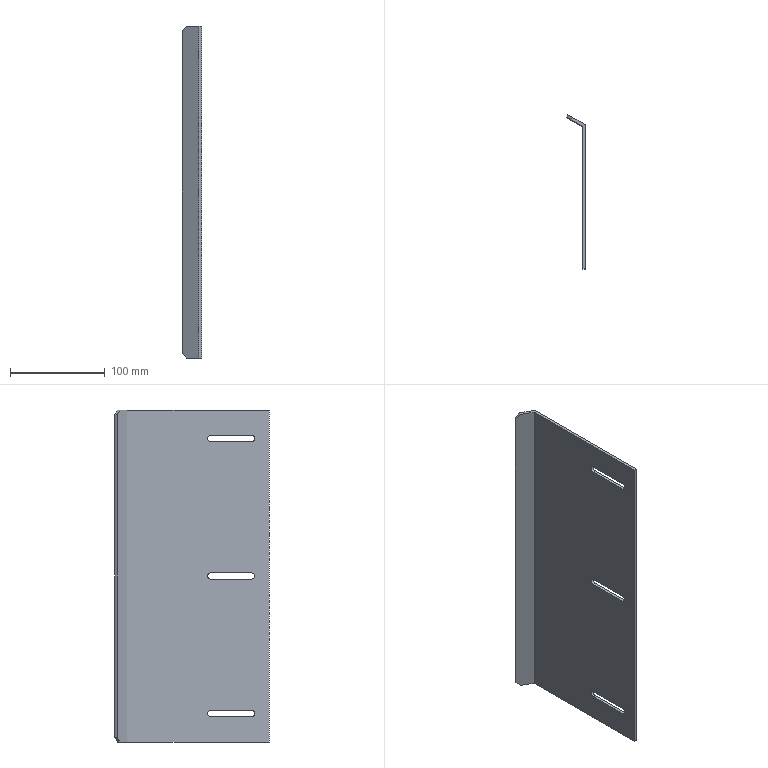Part | SolidWorks | features ICE 3, Fillet 2, Chamfer 1, Extrusion 1 | 1 solid | 24 faces | box 20.321 x 162.598 x 350 mm | volume 177208 mm3 | plane 16 | cylinder 8 | commonest cylinder face diameters 6.5 x6 0.4 x1 6.4 x1
STEP:
#1=CARTESIAN_POINT('',(0.,-150.,350.));
#2=VERTEX_POINT('',#1);
#3=CARTESIAN_POINT('',(3.,-150.,350.));
#4=VERTEX_POINT('',#3);
#5=CARTESIAN_POINT('',(0.,-150.,350.));
#6=DIRECTION('',(1.,0.,0.));
#7=VECTOR('',#6,1000.);
#8=LINE('',#5,#7);
#9=EDGE_CURVE('',#2,#4,#8,.T.);
#10=ORIENTED_EDGE('',*,*,#9,.F.);
#11=CARTESIAN_POINT('',(0.,-150.,0.));
#12=VERTEX_POINT('',#11);
#13=CARTESIAN_POINT('',(0.,-150.,0.));
#14=DIRECTION('',(0.,0.,1.));
#15=VECTOR('',#14,1000.);
#16=LINE('',#13,#15);
#17=EDGE_CURVE('',#12,#2,#16,.T.);
#18=ORIENTED_EDGE('',*,*,#17,.F.);
#19=CARTESIAN_POINT('',(3.,-150.,0.));
#20=VERTEX_POINT('',#19);
#21=CARTESIAN_POINT('',(0.,-150.,0.));
#22=DIRECTION('',(1.,0.,0.));
#23=VECTOR('',#22,1000.);
#24=LINE('',#21,#23);
#25=EDGE_CURVE('',#12,#20,#24,.T.);
#26=ORIENTED_EDGE('',*,*,#25,.T.);
#27=CARTESIAN_POINT('',(3.,-150.,0.));
#28=DIRECTION('',(0.,0.,1.));
#29=VECTOR('',#28,1000.);
#30=LINE('',#27,#29);
#31=EDGE_CURVE('',#20,#4,#30,.T.);
#32=ORIENTED_EDGE('',*,*,#31,.T.);
#33=EDGE_LOOP('',(#10,#18,#26,#32));
#34=FACE_OUTER_BOUND('',#33,.T.);
#35=CARTESIAN_POINT('',(0.,-150.,0.));
#36=DIRECTION('',(0.,-1.,0.));
#37=DIRECTION('',(0.,0.,-1.));
#38=AXIS2_PLACEMENT_3D('',#35,#36,#37);
#39=PLANE('',#38);
#40=ADVANCED_FACE('',(#34),#39,.T.);
#41=CARTESIAN_POINT('',(0.,-131.75,171.75));
#42=VERTEX_POINT('',#41);
#43=CARTESIAN_POINT('',(0.,-131.75,178.25));
#44=VERTEX_POINT('',#43);
#45=CARTESIAN_POINT('',(0.,-131.75,175.));
#46=DIRECTION('',(-1.,0.,0.));
#47=DIRECTION('',(0.,0.,1.));
#48=AXIS2_PLACEMENT_3D('',#45,#46,#47);
#49=CIRCLE('',#48,3.25);
#50=EDGE_CURVE('',#42,#44,#49,.T.);
#51=ORIENTED_EDGE('',*,*,#50,.F.);
#52=CARTESIAN_POINT('',(0.,-88.25,171.75));
#53=VERTEX_POINT('',#52);
#54=CARTESIAN_POINT('',(0.,0.,171.75));
#55=DIRECTION('',(0.,-1.,0.));
#56=VECTOR('',#55,1000.);
#57=LINE('',#54,#56);
#58=EDGE_CURVE('',#53,#42,#57,.T.);
#59=ORIENTED_EDGE('',*,*,#58,.F.);
#60=CARTESIAN_POINT('',(0.,-88.25,178.25));
#61=VERTEX_POINT('',#60);
#62=CARTESIAN_POINT('',(0.,-88.25,175.));
#63=DIRECTION('',(-1.,0.,0.));
#64=DIRECTION('',(0.,0.,1.));
#65=AXIS2_PLACEMENT_3D('',#62,#63,#64);
#66=CIRCLE('',#65,3.25);
#67=EDGE_CURVE('',#61,#53,#66,.T.);
#68=ORIENTED_EDGE('',*,*,#67,.F.);
#69=CARTESIAN_POINT('',(0.,0.,178.25));
#70=DIRECTION('',(0.,1.,0.));
#71=VECTOR('',#70,1000.);
#72=LINE('',#69,#71);
#73=EDGE_CURVE('',#44,#61,#72,.T.);
#74=ORIENTED_EDGE('',*,*,#73,.F.);
#75=EDGE_LOOP('',(#51,#59,#68,#74));
#76=FACE_BOUND('',#75,.T.);
#77=CARTESIAN_POINT('',(0.,-88.25,33.25));
#78=VERTEX_POINT('',#77);
#79=CARTESIAN_POINT('',(0.,-88.25,26.75));
#80=VERTEX_POINT('',#79);
#81=CARTESIAN_POINT('',(0.,-88.25,30.));
#82=DIRECTION('',(-1.,0.,0.));
#83=DIRECTION('',(0.,0.,1.));
#84=AXIS2_PLACEMENT_3D('',#81,#82,#83);
#85=CIRCLE('',#84,3.25);
#86=EDGE_CURVE('',#78,#80,#85,.T.);
#87=ORIENTED_EDGE('',*,*,#86,.F.);
#88=CARTESIAN_POINT('',(0.,-131.75,33.25));
#89=VERTEX_POINT('',#88);
#90=CARTESIAN_POINT('',(0.,-131.75,33.25));
#91=DIRECTION('',(0.,1.,0.));
#92=VECTOR('',#91,1000.);
#93=LINE('',#90,#92);
#94=EDGE_CURVE('',#89,#78,#93,.T.);
#95=ORIENTED_EDGE('',*,*,#94,.F.);
#96=CARTESIAN_POINT('',(0.,-131.75,26.75));
#97=VERTEX_POINT('',#96);
#98=CARTESIAN_POINT('',(0.,-131.75,30.));
#99=DIRECTION('',(-1.,0.,0.));
#100=DIRECTION('',(0.,0.,1.));
#101=AXIS2_PLACEMENT_3D('',#98,#99,#100);
#102=CIRCLE('',#101,3.25);
#103=EDGE_CURVE('',#97,#89,#102,.T.);
#104=ORIENTED_EDGE('',*,*,#103,.F.);
#105=CARTESIAN_POINT('',(0.,-88.25,26.75));
#106=DIRECTION('',(0.,-1.,0.));
#107=VECTOR('',#106,1000.);
#108=LINE('',#105,#107);
#109=EDGE_CURVE('',#80,#97,#108,.T.);
#110=ORIENTED_EDGE('',*,*,#109,.F.);
#111=EDGE_LOOP('',(#87,#95,#104,#110));
#112=FACE_BOUND('',#111,.T.);
#113=CARTESIAN_POINT('',(0.,-88.25,323.25));
#114=VERTEX_POINT('',#113);
#115=CARTESIAN_POINT('',(0.,-88.25,316.75));
#116=VERTEX_POINT('',#115);
#117=CARTESIAN_POINT('',(0.,-88.25,320.));
#118=DIRECTION('',(-1.,0.,0.));
#119=DIRECTION('',(0.,0.,1.));
#120=AXIS2_PLACEMENT_3D('',#117,#118,#119);
#121=CIRCLE('',#120,3.25);
#122=EDGE_CURVE('',#114,#116,#121,.T.);
#123=ORIENTED_EDGE('',*,*,#122,.F.);
#124=CARTESIAN_POINT('',(0.,-131.75,323.25));
#125=VERTEX_POINT('',#124);
#126=CARTESIAN_POINT('',(0.,-131.75,323.25));
#127=DIRECTION('',(0.,1.,0.));
#128=VECTOR('',#127,1000.);
#129=LINE('',#126,#128);
#130=EDGE_CURVE('',#125,#114,#129,.T.);
#131=ORIENTED_EDGE('',*,*,#130,.F.);
#132=CARTESIAN_POINT('',(0.,-131.75,316.75));
#133=VERTEX_POINT('',#132);
#134=CARTESIAN_POINT('',(0.,-131.75,320.));
#135=DIRECTION('',(-1.,0.,0.));
#136=DIRECTION('',(0.,0.,1.));
#137=AXIS2_PLACEMENT_3D('',#134,#135,#136);
#138=CIRCLE('',#137,3.25);
#139=EDGE_CURVE('',#133,#125,#138,.T.);
#140=ORIENTED_EDGE('',*,*,#139,.F.);
#141=CARTESIAN_POINT('',(0.,-88.25,316.75));
#142=DIRECTION('',(0.,-1.,0.));
#143=VECTOR('',#142,1000.);
#144=LINE('',#141,#143);
#145=EDGE_CURVE('',#116,#133,#144,.T.);
#146=ORIENTED_EDGE('',*,*,#145,.F.);
#147=EDGE_LOOP('',(#123,#131,#140,#146));
#148=FACE_BOUND('',#147,.T.);
#149=CARTESIAN_POINT('',(0.,-0.1155,350.));
#150=VERTEX_POINT('',#149);
#151=CARTESIAN_POINT('',(0.,0.,350.));
#152=DIRECTION('',(0.,-1.,0.));
#153=VECTOR('',#152,1000.);
#154=LINE('',#151,#153);
#155=EDGE_CURVE('',#150,#2,#154,.T.);
#156=ORIENTED_EDGE('',*,*,#155,.F.);
#157=CARTESIAN_POINT('',(0.,-0.1155,0.));
#158=VERTEX_POINT('',#157);
#159=CARTESIAN_POINT('',(0.,-0.1155,0.));
#160=DIRECTION('',(0.,0.,-1.));
#161=VECTOR('',#160,1000.);
#162=LINE('',#159,#161);
#163=EDGE_CURVE('',#150,#158,#162,.T.);
#164=ORIENTED_EDGE('',*,*,#163,.T.);
#165=CARTESIAN_POINT('',(0.,0.,0.));
#166=DIRECTION('',(0.,-1.,0.));
#167=VECTOR('',#166,1000.);
#168=LINE('',#165,#167);
#169=EDGE_CURVE('',#158,#12,#168,.T.);
#170=ORIENTED_EDGE('',*,*,#169,.T.);
#171=ORIENTED_EDGE('',*,*,#17,.T.);
#172=EDGE_LOOP('',(#156,#164,#170,#171));
#173=FACE_OUTER_BOUND('',#172,.T.);
#174=CARTESIAN_POINT('',(0.,0.,0.));
#175=DIRECTION('',(-1.,0.,0.));
#176=DIRECTION('',(0.,0.,1.));
#177=AXIS2_PLACEMENT_3D('',#174,#175,#176);
#178=PLANE('',#177);
#179=ADVANCED_FACE('',(#76,#112,#148,#173),#178,.T.);
#180=CARTESIAN_POINT('',(-12.99,7.5,0.));
#181=VERTEX_POINT('',#180);
#182=CARTESIAN_POINT('',(-0.1,0.05774,0.));
#183=VERTEX_POINT('',#182);
#184=CARTESIAN_POINT('',(-17.321,10.,0.));
#185=DIRECTION('',(0.866,-0.5,0.));
#186=VECTOR('',#185,1000.);
#187=LINE('',#184,#186);
#188=EDGE_CURVE('',#181,#183,#187,.T.);
#189=ORIENTED_EDGE('',*,*,#188,.T.);
#190=CARTESIAN_POINT('',(-0.1,0.05774,350.));
#191=VERTEX_POINT('',#190);
#192=CARTESIAN_POINT('',(-0.1,0.05774,350.));
#193=DIRECTION('',(0.,0.,1.));
#194=VECTOR('',#193,1000.);
#195=LINE('',#192,#194);
#196=EDGE_CURVE('',#183,#191,#195,.T.);
#197=ORIENTED_EDGE('',*,*,#196,.T.);
#198=CARTESIAN_POINT('',(-12.99,7.5,350.));
#199=VERTEX_POINT('',#198);
#200=CARTESIAN_POINT('',(-17.321,10.,350.));
#201=DIRECTION('',(0.866,-0.5,0.));
#202=VECTOR('',#201,1000.);
#203=LINE('',#200,#202);
#204=EDGE_CURVE('',#199,#191,#203,.T.);
#205=ORIENTED_EDGE('',*,*,#204,.F.);
#206=CARTESIAN_POINT('',(-17.321,10.,345.));
#207=VERTEX_POINT('',#206);
#208=CARTESIAN_POINT('',(-166.71,96.25,172.5));
#209=DIRECTION('',(-0.6124,0.3536,-0.7071));
#210=VECTOR('',#209,1000.);
#211=LINE('',#208,#210);
#212=EDGE_CURVE('',#199,#207,#211,.T.);
#213=ORIENTED_EDGE('',*,*,#212,.T.);
#214=CARTESIAN_POINT('',(-17.321,10.,5.));
#215=VERTEX_POINT('',#214);
#216=CARTESIAN_POINT('',(-17.321,10.,0.));
#217=DIRECTION('',(0.,0.,1.));
#218=VECTOR('',#217,1000.);
#219=LINE('',#216,#218);
#220=EDGE_CURVE('',#215,#207,#219,.T.);
#221=ORIENTED_EDGE('',*,*,#220,.F.);
#222=CARTESIAN_POINT('',(-15.155,8.75,2.5));
#223=DIRECTION('',(0.6124,-0.3536,-0.7071));
#224=VECTOR('',#223,1000.);
#225=LINE('',#222,#224);
#226=EDGE_CURVE('',#215,#181,#225,.T.);
#227=ORIENTED_EDGE('',*,*,#226,.T.);
#228=EDGE_LOOP('',(#189,#197,#205,#213,#221,#227));
#229=FACE_OUTER_BOUND('',#228,.T.);
#230=CARTESIAN_POINT('',(-17.321,10.,0.));
#231=DIRECTION('',(-0.5,-0.866,0.));
#232=DIRECTION('',(0.866,-0.5,0.));
#233=AXIS2_PLACEMENT_3D('',#230,#231,#232);
#234=PLANE('',#233);
#235=ADVANCED_FACE('',(#229),#234,.T.);
#236=CARTESIAN_POINT('',(-15.821,12.598,5.));
#237=VERTEX_POINT('',#236);
#238=CARTESIAN_POINT('',(-15.821,12.598,345.));
#239=VERTEX_POINT('',#238);
#240=CARTESIAN_POINT('',(-15.821,12.598,0.));
#241=DIRECTION('',(0.,0.,1.));
#242=VECTOR('',#241,1000.);
#243=LINE('',#240,#242);
#244=EDGE_CURVE('',#237,#239,#243,.T.);
#245=ORIENTED_EDGE('',*,*,#244,.F.);
#246=CARTESIAN_POINT('',(-17.321,10.,5.));
#247=DIRECTION('',(-0.5,-0.866,0.));
#248=VECTOR('',#247,1000.);
#249=LINE('',#246,#248);
#250=EDGE_CURVE('',#237,#215,#249,.T.);
#251=ORIENTED_EDGE('',*,*,#250,.T.);
#252=ORIENTED_EDGE('',*,*,#220,.T.);
#253=CARTESIAN_POINT('',(-15.821,12.598,345.));
#254=DIRECTION('',(0.5,0.866,0.));
#255=VECTOR('',#254,1000.);
#256=LINE('',#253,#255);
#257=EDGE_CURVE('',#207,#239,#256,.T.);
#258=ORIENTED_EDGE('',*,*,#257,.T.);
#259=EDGE_LOOP('',(#245,#251,#252,#258));
#260=FACE_OUTER_BOUND('',#259,.T.);
#261=CARTESIAN_POINT('',(-15.821,12.598,0.));
#262=DIRECTION('',(-0.866,0.5,0.));
#263=DIRECTION('',(-0.5,-0.866,0.));
#264=AXIS2_PLACEMENT_3D('',#261,#262,#263);
#265=PLANE('',#264);
#266=ADVANCED_FACE('',(#260),#265,.T.);
#267=CARTESIAN_POINT('',(1.4,2.656,350.));
#268=VERTEX_POINT('',#267);
#269=CARTESIAN_POINT('',(-11.49,10.098,350.));
#270=VERTEX_POINT('',#269);
#271=CARTESIAN_POINT('',(3.,1.732,350.));
#272=DIRECTION('',(-0.866,0.5,0.));
#273=VECTOR('',#272,1000.);
#274=LINE('',#271,#273);
#275=EDGE_CURVE('',#268,#270,#274,.T.);
#276=ORIENTED_EDGE('',*,*,#275,.F.);
#277=CARTESIAN_POINT('',(1.4,2.656,0.));
#278=VERTEX_POINT('',#277);
#279=CARTESIAN_POINT('',(1.4,2.656,0.));
#280=DIRECTION('',(0.,0.,-1.));
#281=VECTOR('',#280,1000.);
#282=LINE('',#279,#281);
#283=EDGE_CURVE('',#268,#278,#282,.T.);
#284=ORIENTED_EDGE('',*,*,#283,.T.);
#285=CARTESIAN_POINT('',(-11.49,10.098,0.));
#286=VERTEX_POINT('',#285);
#287=CARTESIAN_POINT('',(3.,1.732,0.));
#288=DIRECTION('',(-0.866,0.5,0.));
#289=VECTOR('',#288,1000.);
#290=LINE('',#287,#289);
#291=EDGE_CURVE('',#278,#286,#290,.T.);
#292=ORIENTED_EDGE('',*,*,#291,.T.);
#293=CARTESIAN_POINT('',(-4.245,5.915,-8.366));
#294=DIRECTION('',(-0.6124,0.3536,0.7071));
#295=VECTOR('',#294,1000.);
#296=LINE('',#293,#295);
#297=EDGE_CURVE('',#286,#237,#296,.T.);
#298=ORIENTED_EDGE('',*,*,#297,.T.);
#299=ORIENTED_EDGE('',*,*,#244,.T.);
#300=CARTESIAN_POINT('',(-155.8,93.415,183.366));
#301=DIRECTION('',(0.6124,-0.3536,0.7071));
#302=VECTOR('',#301,1000.);
#303=LINE('',#300,#302);
#304=EDGE_CURVE('',#239,#270,#303,.T.);
#305=ORIENTED_EDGE('',*,*,#304,.T.);
#306=EDGE_LOOP('',(#276,#284,#292,#298,#299,#305));
#307=FACE_OUTER_BOUND('',#306,.T.);
#308=CARTESIAN_POINT('',(3.,1.732,0.));
#309=DIRECTION('',(0.5,0.866,0.));
#310=DIRECTION('',(-0.866,0.5,0.));
#311=AXIS2_PLACEMENT_3D('',#308,#309,#310);
#312=PLANE('',#311);
#313=ADVANCED_FACE('',(#307),#312,.T.);
#314=CARTESIAN_POINT('',(3.,-131.75,178.25));
#315=VERTEX_POINT('',#314);
#316=CARTESIAN_POINT('',(3.,-131.75,171.75));
#317=VERTEX_POINT('',#316);
#318=CARTESIAN_POINT('',(3.,-131.75,175.));
#319=DIRECTION('',(1.,0.,0.));
#320=DIRECTION('',(0.,0.,-1.));
#321=AXIS2_PLACEMENT_3D('',#318,#319,#320);
#322=CIRCLE('',#321,3.25);
#323=EDGE_CURVE('',#315,#317,#322,.T.);
#324=ORIENTED_EDGE('',*,*,#323,.F.);
#325=CARTESIAN_POINT('',(3.,-88.25,178.25));
#326=VERTEX_POINT('',#325);
#327=CARTESIAN_POINT('',(3.,-88.25,178.25));
#328=DIRECTION('',(0.,-1.,0.));
#329=VECTOR('',#328,1000.);
#330=LINE('',#327,#329);
#331=EDGE_CURVE('',#326,#315,#330,.T.);
#332=ORIENTED_EDGE('',*,*,#331,.F.);
#333=CARTESIAN_POINT('',(3.,-88.25,171.75));
#334=VERTEX_POINT('',#333);
#335=CARTESIAN_POINT('',(3.,-88.25,175.));
#336=DIRECTION('',(1.,0.,0.));
#337=DIRECTION('',(0.,0.,-1.));
#338=AXIS2_PLACEMENT_3D('',#335,#336,#337);
#339=CIRCLE('',#338,3.25);
#340=EDGE_CURVE('',#334,#326,#339,.T.);
#341=ORIENTED_EDGE('',*,*,#340,.F.);
#342=CARTESIAN_POINT('',(3.,-131.75,171.75));
#343=DIRECTION('',(0.,1.,0.));
#344=VECTOR('',#343,1000.);
#345=LINE('',#342,#344);
#346=EDGE_CURVE('',#317,#334,#345,.T.);
#347=ORIENTED_EDGE('',*,*,#346,.F.);
#348=EDGE_LOOP('',(#324,#332,#341,#347));
#349=FACE_BOUND('',#348,.T.);
#350=CARTESIAN_POINT('',(3.,-88.25,33.25));
#351=VERTEX_POINT('',#350);
#352=CARTESIAN_POINT('',(3.,-88.25,26.75));
#353=VERTEX_POINT('',#352);
#354=CARTESIAN_POINT('',(3.,-88.25,30.));
#355=DIRECTION('',(-1.,0.,0.));
#356=DIRECTION('',(0.,0.,1.));
#357=AXIS2_PLACEMENT_3D('',#354,#355,#356);
#358=CIRCLE('',#357,3.25);
#359=EDGE_CURVE('',#351,#353,#358,.T.);
#360=ORIENTED_EDGE('',*,*,#359,.T.);
#361=CARTESIAN_POINT('',(3.,-131.75,26.75));
#362=VERTEX_POINT('',#361);
#363=CARTESIAN_POINT('',(3.,-88.25,26.75));
#364=DIRECTION('',(0.,-1.,0.));
#365=VECTOR('',#364,1000.);
#366=LINE('',#363,#365);
#367=EDGE_CURVE('',#353,#362,#366,.T.);
#368=ORIENTED_EDGE('',*,*,#367,.T.);
#369=CARTESIAN_POINT('',(3.,-131.75,33.25));
#370=VERTEX_POINT('',#369);
#371=CARTESIAN_POINT('',(3.,-131.75,30.));
#372=DIRECTION('',(-1.,0.,0.));
#373=DIRECTION('',(0.,0.,1.));
#374=AXIS2_PLACEMENT_3D('',#371,#372,#373);
#375=CIRCLE('',#374,3.25);
#376=EDGE_CURVE('',#362,#370,#375,.T.);
#377=ORIENTED_EDGE('',*,*,#376,.T.);
#378=CARTESIAN_POINT('',(3.,-131.75,33.25));
#379=DIRECTION('',(0.,1.,0.));
#380=VECTOR('',#379,1000.);
#381=LINE('',#378,#380);
#382=EDGE_CURVE('',#370,#351,#381,.T.);
#383=ORIENTED_EDGE('',*,*,#382,.T.);
#384=EDGE_LOOP('',(#360,#368,#377,#383));
#385=FACE_BOUND('',#384,.T.);
#386=CARTESIAN_POINT('',(3.,-88.25,323.25));
#387=VERTEX_POINT('',#386);
#388=CARTESIAN_POINT('',(3.,-88.25,316.75));
#389=VERTEX_POINT('',#388);
#390=CARTESIAN_POINT('',(3.,-88.25,320.));
#391=DIRECTION('',(-1.,0.,0.));
#392=DIRECTION('',(0.,0.,1.));
#393=AXIS2_PLACEMENT_3D('',#390,#391,#392);
#394=CIRCLE('',#393,3.25);
#395=EDGE_CURVE('',#387,#389,#394,.T.);
#396=ORIENTED_EDGE('',*,*,#395,.T.);
#397=CARTESIAN_POINT('',(3.,-131.75,316.75));
#398=VERTEX_POINT('',#397);
#399=CARTESIAN_POINT('',(3.,-88.25,316.75));
#400=DIRECTION('',(0.,-1.,0.));
#401=VECTOR('',#400,1000.);
#402=LINE('',#399,#401);
#403=EDGE_CURVE('',#389,#398,#402,.T.);
#404=ORIENTED_EDGE('',*,*,#403,.T.);
#405=CARTESIAN_POINT('',(3.,-131.75,323.25));
#406=VERTEX_POINT('',#405);
#407=CARTESIAN_POINT('',(3.,-131.75,320.));
#408=DIRECTION('',(-1.,0.,0.));
#409=DIRECTION('',(0.,0.,1.));
#410=AXIS2_PLACEMENT_3D('',#407,#408,#409);
#411=CIRCLE('',#410,3.25);
#412=EDGE_CURVE('',#398,#406,#411,.T.);
#413=ORIENTED_EDGE('',*,*,#412,.T.);
#414=CARTESIAN_POINT('',(3.,-131.75,323.25));
#415=DIRECTION('',(0.,1.,0.));
#416=VECTOR('',#415,1000.);
#417=LINE('',#414,#416);
#418=EDGE_CURVE('',#406,#387,#417,.T.);
#419=ORIENTED_EDGE('',*,*,#418,.T.);
#420=EDGE_LOOP('',(#396,#404,#413,#419));
#421=FACE_BOUND('',#420,.T.);
#422=CARTESIAN_POINT('',(3.,-0.1155,0.));
#423=VERTEX_POINT('',#422);
#424=CARTESIAN_POINT('',(3.,-150.,0.));
#425=DIRECTION('',(0.,1.,0.));
#426=VECTOR('',#425,1000.);
#427=LINE('',#424,#426);
#428=EDGE_CURVE('',#20,#423,#427,.T.);
#429=ORIENTED_EDGE('',*,*,#428,.T.);
#430=CARTESIAN_POINT('',(3.,-0.1155,350.));
#431=VERTEX_POINT('',#430);
#432=CARTESIAN_POINT('',(3.,-0.1155,0.));
#433=DIRECTION('',(0.,0.,1.));
#434=VECTOR('',#433,1000.);
#435=LINE('',#432,#434);
#436=EDGE_CURVE('',#423,#431,#435,.T.);
#437=ORIENTED_EDGE('',*,*,#436,.T.);
#438=CARTESIAN_POINT('',(3.,-150.,350.));
#439=DIRECTION('',(0.,1.,0.));
#440=VECTOR('',#439,1000.);
#441=LINE('',#438,#440);
#442=EDGE_CURVE('',#4,#431,#441,.T.);
#443=ORIENTED_EDGE('',*,*,#442,.F.);
#444=ORIENTED_EDGE('',*,*,#31,.F.);
#445=EDGE_LOOP('',(#429,#437,#443,#444));
#446=FACE_OUTER_BOUND('',#445,.T.);
#447=CARTESIAN_POINT('',(3.,-150.,0.));
#448=DIRECTION('',(1.,0.,0.));
#449=DIRECTION('',(0.,0.,-1.));
#450=AXIS2_PLACEMENT_3D('',#447,#448,#449);
#451=PLANE('',#450);
#452=ADVANCED_FACE('',(#349,#385,#421,#446),#451,.T.);
#453=ORIENTED_EDGE('',*,*,#291,.F.);
#454=CARTESIAN_POINT('',(-0.2,-0.1155,0.));
#455=DIRECTION('',(0.,0.,-1.));
#456=DIRECTION('',(1.,0.,0.));
#457=AXIS2_PLACEMENT_3D('',#454,#455,#456);
#458=CIRCLE('',#457,3.2);
#459=EDGE_CURVE('',#278,#423,#458,.T.);
#460=ORIENTED_EDGE('',*,*,#459,.T.);
#461=ORIENTED_EDGE('',*,*,#428,.F.);
#462=ORIENTED_EDGE('',*,*,#25,.F.);
#463=ORIENTED_EDGE('',*,*,#169,.F.);
#464=CARTESIAN_POINT('',(-0.2,-0.1155,0.));
#465=DIRECTION('',(0.,0.,1.));
#466=DIRECTION('',(1.,0.,0.));
#467=AXIS2_PLACEMENT_3D('',#464,#465,#466);
#468=CIRCLE('',#467,0.2);
#469=EDGE_CURVE('',#158,#183,#468,.T.);
#470=ORIENTED_EDGE('',*,*,#469,.T.);
#471=ORIENTED_EDGE('',*,*,#188,.F.);
#472=CARTESIAN_POINT('',(-11.49,10.098,0.));
#473=DIRECTION('',(0.5,0.866,0.));
#474=VECTOR('',#473,1000.);
#475=LINE('',#472,#474);
#476=EDGE_CURVE('',#181,#286,#475,.T.);
#477=ORIENTED_EDGE('',*,*,#476,.T.);
#478=EDGE_LOOP('',(#453,#460,#461,#462,#463,#470,#471,#477));
#479=FACE_OUTER_BOUND('',#478,.T.);
#480=CARTESIAN_POINT('',(0.,0.,0.));
#481=DIRECTION('',(0.,0.,1.));
#482=DIRECTION('',(1.,0.,0.));
#483=AXIS2_PLACEMENT_3D('',#480,#481,#482);
#484=PLANE('',#483);
#485=ADVANCED_FACE('',(#479),#484,.F.);
#486=ORIENTED_EDGE('',*,*,#442,.T.);
#487=CARTESIAN_POINT('',(-0.2,-0.1155,350.));
#488=DIRECTION('',(0.,0.,1.));
#489=DIRECTION('',(1.,0.,0.));
#490=AXIS2_PLACEMENT_3D('',#487,#488,#489);
#491=CIRCLE('',#490,3.2);
#492=EDGE_CURVE('',#431,#268,#491,.T.);
#493=ORIENTED_EDGE('',*,*,#492,.T.);
#494=ORIENTED_EDGE('',*,*,#275,.T.);
#495=CARTESIAN_POINT('',(-12.99,7.5,350.));
#496=DIRECTION('',(-0.5,-0.866,0.));
#497=VECTOR('',#496,1000.);
#498=LINE('',#495,#497);
#499=EDGE_CURVE('',#270,#199,#498,.T.);
#500=ORIENTED_EDGE('',*,*,#499,.T.);
#501=ORIENTED_EDGE('',*,*,#204,.T.);
#502=CARTESIAN_POINT('',(-0.2,-0.1155,350.));
#503=DIRECTION('',(0.,0.,-1.));
#504=DIRECTION('',(1.,0.,0.));
#505=AXIS2_PLACEMENT_3D('',#502,#503,#504);
#506=CIRCLE('',#505,0.2);
#507=EDGE_CURVE('',#191,#150,#506,.T.);
#508=ORIENTED_EDGE('',*,*,#507,.T.);
#509=ORIENTED_EDGE('',*,*,#155,.T.);
#510=ORIENTED_EDGE('',*,*,#9,.T.);
#511=EDGE_LOOP('',(#486,#493,#494,#500,#501,#508,#509,#510));
#512=FACE_OUTER_BOUND('',#511,.T.);
#513=CARTESIAN_POINT('',(0.,0.,350.));
#514=DIRECTION('',(0.,0.,1.));
#515=DIRECTION('',(1.,0.,0.));
#516=AXIS2_PLACEMENT_3D('',#513,#514,#515);
#517=PLANE('',#516);
#518=ADVANCED_FACE('',(#512),#517,.T.);
#519=ORIENTED_EDGE('',*,*,#122,.T.);
#520=CARTESIAN_POINT('',(3.,-88.25,316.75));
#521=DIRECTION('',(-1.,0.,0.));
#522=VECTOR('',#521,1000.);
#523=LINE('',#520,#522);
#524=EDGE_CURVE('',#389,#116,#523,.T.);
#525=ORIENTED_EDGE('',*,*,#524,.F.);
#526=ORIENTED_EDGE('',*,*,#395,.F.);
#527=CARTESIAN_POINT('',(3.,-88.25,323.25));
#528=DIRECTION('',(-1.,0.,0.));
#529=VECTOR('',#528,1000.);
#530=LINE('',#527,#529);
#531=EDGE_CURVE('',#387,#114,#530,.T.);
#532=ORIENTED_EDGE('',*,*,#531,.T.);
#533=EDGE_LOOP('',(#519,#525,#526,#532));
#534=FACE_OUTER_BOUND('',#533,.T.);
#535=CARTESIAN_POINT('',(3.,-88.25,320.));
#536=DIRECTION('',(-1.,0.,0.));
#537=DIRECTION('',(0.,0.,1.));
#538=AXIS2_PLACEMENT_3D('',#535,#536,#537);
#539=CYLINDRICAL_SURFACE('',#538,3.25);
#540=ADVANCED_FACE('',(#534),#539,.F.);
#541=ORIENTED_EDGE('',*,*,#130,.T.);
#542=ORIENTED_EDGE('',*,*,#531,.F.);
#543=ORIENTED_EDGE('',*,*,#418,.F.);
#544=CARTESIAN_POINT('',(3.,-131.75,323.25));
#545=DIRECTION('',(-1.,0.,0.));
#546=VECTOR('',#545,1000.);
#547=LINE('',#544,#546);
#548=EDGE_CURVE('',#406,#125,#547,.T.);
#549=ORIENTED_EDGE('',*,*,#548,.T.);
#550=EDGE_LOOP('',(#541,#542,#543,#549));
#551=FACE_OUTER_BOUND('',#550,.T.);
#552=CARTESIAN_POINT('',(3.,-131.75,323.25));
#553=DIRECTION('',(0.,0.,1.));
#554=DIRECTION('',(1.,0.,0.));
#555=AXIS2_PLACEMENT_3D('',#552,#553,#554);
#556=PLANE('',#555);
#557=ADVANCED_FACE('',(#551),#556,.F.);
#558=ORIENTED_EDGE('',*,*,#139,.T.);
#559=ORIENTED_EDGE('',*,*,#548,.F.);
#560=ORIENTED_EDGE('',*,*,#412,.F.);
#561=CARTESIAN_POINT('',(3.,-131.75,316.75));
#562=DIRECTION('',(-1.,0.,0.));
#563=VECTOR('',#562,1000.);
#564=LINE('',#561,#563);
#565=EDGE_CURVE('',#398,#133,#564,.T.);
#566=ORIENTED_EDGE('',*,*,#565,.T.);
#567=EDGE_LOOP('',(#558,#559,#560,#566));
#568=FACE_OUTER_BOUND('',#567,.T.);
#569=CARTESIAN_POINT('',(3.,-131.75,320.));
#570=DIRECTION('',(-1.,0.,0.));
#571=DIRECTION('',(0.,0.,1.));
#572=AXIS2_PLACEMENT_3D('',#569,#570,#571);
#573=CYLINDRICAL_SURFACE('',#572,3.25);
#574=ADVANCED_FACE('',(#568),#573,.F.);
#575=ORIENTED_EDGE('',*,*,#145,.T.);
#576=ORIENTED_EDGE('',*,*,#565,.F.);
#577=ORIENTED_EDGE('',*,*,#403,.F.);
#578=ORIENTED_EDGE('',*,*,#524,.T.);
#579=EDGE_LOOP('',(#575,#576,#577,#578));
#580=FACE_OUTER_BOUND('',#579,.T.);
#581=CARTESIAN_POINT('',(3.,-88.25,316.75));
#582=DIRECTION('',(0.,0.,-1.));
#583=DIRECTION('',(-1.,0.,0.));
#584=AXIS2_PLACEMENT_3D('',#581,#582,#583);
#585=PLANE('',#584);
#586=ADVANCED_FACE('',(#580),#585,.F.);
#587=ORIENTED_EDGE('',*,*,#86,.T.);
#588=CARTESIAN_POINT('',(3.,-88.25,26.75));
#589=DIRECTION('',(-1.,0.,0.));
#590=VECTOR('',#589,1000.);
#591=LINE('',#588,#590);
#592=EDGE_CURVE('',#353,#80,#591,.T.);
#593=ORIENTED_EDGE('',*,*,#592,.F.);
#594=ORIENTED_EDGE('',*,*,#359,.F.);
#595=CARTESIAN_POINT('',(3.,-88.25,33.25));
#596=DIRECTION('',(-1.,0.,0.));
#597=VECTOR('',#596,1000.);
#598=LINE('',#595,#597);
#599=EDGE_CURVE('',#351,#78,#598,.T.);
#600=ORIENTED_EDGE('',*,*,#599,.T.);
#601=EDGE_LOOP('',(#587,#593,#594,#600));
#602=FACE_OUTER_BOUND('',#601,.T.);
#603=CARTESIAN_POINT('',(3.,-88.25,30.));
#604=DIRECTION('',(-1.,0.,0.));
#605=DIRECTION('',(0.,0.,1.));
#606=AXIS2_PLACEMENT_3D('',#603,#604,#605);
#607=CYLINDRICAL_SURFACE('',#606,3.25);
#608=ADVANCED_FACE('',(#602),#607,.F.);
#609=ORIENTED_EDGE('',*,*,#94,.T.);
#610=ORIENTED_EDGE('',*,*,#599,.F.);
#611=ORIENTED_EDGE('',*,*,#382,.F.);
#612=CARTESIAN_POINT('',(3.,-131.75,33.25));
#613=DIRECTION('',(-1.,0.,0.));
#614=VECTOR('',#613,1000.);
#615=LINE('',#612,#614);
#616=EDGE_CURVE('',#370,#89,#615,.T.);
#617=ORIENTED_EDGE('',*,*,#616,.T.);
#618=EDGE_LOOP('',(#609,#610,#611,#617));
#619=FACE_OUTER_BOUND('',#618,.T.);
#620=CARTESIAN_POINT('',(3.,-131.75,33.25));
#621=DIRECTION('',(0.,0.,1.));
#622=DIRECTION('',(1.,0.,0.));
#623=AXIS2_PLACEMENT_3D('',#620,#621,#622);
#624=PLANE('',#623);
#625=ADVANCED_FACE('',(#619),#624,.F.);
#626=ORIENTED_EDGE('',*,*,#103,.T.);
#627=ORIENTED_EDGE('',*,*,#616,.F.);
#628=ORIENTED_EDGE('',*,*,#376,.F.);
#629=CARTESIAN_POINT('',(3.,-131.75,26.75));
#630=DIRECTION('',(-1.,0.,0.));
#631=VECTOR('',#630,1000.);
#632=LINE('',#629,#631);
#633=EDGE_CURVE('',#362,#97,#632,.T.);
#634=ORIENTED_EDGE('',*,*,#633,.T.);
#635=EDGE_LOOP('',(#626,#627,#628,#634));
#636=FACE_OUTER_BOUND('',#635,.T.);
#637=CARTESIAN_POINT('',(3.,-131.75,30.));
#638=DIRECTION('',(-1.,0.,0.));
#639=DIRECTION('',(0.,0.,1.));
#640=AXIS2_PLACEMENT_3D('',#637,#638,#639);
#641=CYLINDRICAL_SURFACE('',#640,3.25);
#642=ADVANCED_FACE('',(#636),#641,.F.);
#643=ORIENTED_EDGE('',*,*,#109,.T.);
#644=ORIENTED_EDGE('',*,*,#633,.F.);
#645=ORIENTED_EDGE('',*,*,#367,.F.);
#646=ORIENTED_EDGE('',*,*,#592,.T.);
#647=EDGE_LOOP('',(#643,#644,#645,#646));
#648=FACE_OUTER_BOUND('',#647,.T.);
#649=CARTESIAN_POINT('',(3.,-88.25,26.75));
#650=DIRECTION('',(0.,0.,-1.));
#651=DIRECTION('',(-1.,0.,0.));
#652=AXIS2_PLACEMENT_3D('',#649,#650,#651);
#653=PLANE('',#652);
#654=ADVANCED_FACE('',(#648),#653,.F.);
#655=ORIENTED_EDGE('',*,*,#50,.T.);
#656=CARTESIAN_POINT('',(-17.321,-131.75,178.25));
#657=DIRECTION('',(1.,0.,0.));
#658=VECTOR('',#657,1000.);
#659=LINE('',#656,#658);
#660=EDGE_CURVE('',#44,#315,#659,.T.);
#661=ORIENTED_EDGE('',*,*,#660,.T.);
#662=ORIENTED_EDGE('',*,*,#323,.T.);
#663=CARTESIAN_POINT('',(-17.321,-131.75,171.75));
#664=DIRECTION('',(1.,0.,0.));
#665=VECTOR('',#664,1000.);
#666=LINE('',#663,#665);
#667=EDGE_CURVE('',#42,#317,#666,.T.);
#668=ORIENTED_EDGE('',*,*,#667,.F.);
#669=EDGE_LOOP('',(#655,#661,#662,#668));
#670=FACE_OUTER_BOUND('',#669,.T.);
#671=CARTESIAN_POINT('',(-17.321,-131.75,175.));
#672=DIRECTION('',(1.,0.,0.));
#673=DIRECTION('',(0.,0.,-1.));
#674=AXIS2_PLACEMENT_3D('',#671,#672,#673);
#675=CYLINDRICAL_SURFACE('',#674,3.25);
#676=ADVANCED_FACE('',(#670),#675,.F.);
#677=ORIENTED_EDGE('',*,*,#73,.T.);
#678=CARTESIAN_POINT('',(-17.321,-88.25,178.25));
#679=DIRECTION('',(1.,0.,0.));
#680=VECTOR('',#679,1000.);
#681=LINE('',#678,#680);
#682=EDGE_CURVE('',#61,#326,#681,.T.);
#683=ORIENTED_EDGE('',*,*,#682,.T.);
#684=ORIENTED_EDGE('',*,*,#331,.T.);
#685=ORIENTED_EDGE('',*,*,#660,.F.);
#686=EDGE_LOOP('',(#677,#683,#684,#685));
#687=FACE_OUTER_BOUND('',#686,.T.);
#688=CARTESIAN_POINT('',(-17.321,-88.25,178.25));
#689=DIRECTION('',(0.,0.,1.));
#690=DIRECTION('',(1.,0.,0.));
#691=AXIS2_PLACEMENT_3D('',#688,#689,#690);
#692=PLANE('',#691);
#693=ADVANCED_FACE('',(#687),#692,.F.);
#694=ORIENTED_EDGE('',*,*,#67,.T.);
#695=CARTESIAN_POINT('',(-17.321,-88.25,171.75));
#696=DIRECTION('',(1.,0.,0.));
#697=VECTOR('',#696,1000.);
#698=LINE('',#695,#697);
#699=EDGE_CURVE('',#53,#334,#698,.T.);
#700=ORIENTED_EDGE('',*,*,#699,.T.);
#701=ORIENTED_EDGE('',*,*,#340,.T.);
#702=ORIENTED_EDGE('',*,*,#682,.F.);
#703=EDGE_LOOP('',(#694,#700,#701,#702));
#704=FACE_OUTER_BOUND('',#703,.T.);
#705=CARTESIAN_POINT('',(-17.321,-88.25,175.));
#706=DIRECTION('',(1.,0.,0.));
#707=DIRECTION('',(0.,0.,-1.));
#708=AXIS2_PLACEMENT_3D('',#705,#706,#707);
#709=CYLINDRICAL_SURFACE('',#708,3.25);
#710=ADVANCED_FACE('',(#704),#709,.F.);
#711=ORIENTED_EDGE('',*,*,#58,.T.);
#712=ORIENTED_EDGE('',*,*,#667,.T.);
#713=ORIENTED_EDGE('',*,*,#346,.T.);
#714=ORIENTED_EDGE('',*,*,#699,.F.);
#715=EDGE_LOOP('',(#711,#712,#713,#714));
#716=FACE_OUTER_BOUND('',#715,.T.);
#717=CARTESIAN_POINT('',(-17.321,-131.75,171.75));
#718=DIRECTION('',(0.,0.,-1.));
#719=DIRECTION('',(-1.,0.,0.));
#720=AXIS2_PLACEMENT_3D('',#717,#718,#719);
#721=PLANE('',#720);
#722=ADVANCED_FACE('',(#716),#721,.F.);
#723=ORIENTED_EDGE('',*,*,#297,.F.);
#724=ORIENTED_EDGE('',*,*,#476,.F.);
#725=ORIENTED_EDGE('',*,*,#226,.F.);
#726=ORIENTED_EDGE('',*,*,#250,.F.);
#727=EDGE_LOOP('',(#723,#724,#725,#726));
#728=FACE_OUTER_BOUND('',#727,.T.);
#729=CARTESIAN_POINT('',(-15.821,12.598,5.));
#730=DIRECTION('',(-0.6124,0.3536,-0.7071));
#731=DIRECTION('',(0.5,0.866,0.));
#732=AXIS2_PLACEMENT_3D('',#729,#730,#731);
#733=PLANE('',#732);
#734=ADVANCED_FACE('',(#728),#733,.T.);
#735=ORIENTED_EDGE('',*,*,#304,.F.);
#736=ORIENTED_EDGE('',*,*,#257,.F.);
#737=ORIENTED_EDGE('',*,*,#212,.F.);
#738=ORIENTED_EDGE('',*,*,#499,.F.);
#739=EDGE_LOOP('',(#735,#736,#737,#738));
#740=FACE_OUTER_BOUND('',#739,.T.);
#741=CARTESIAN_POINT('',(-12.99,7.5,350.));
#742=DIRECTION('',(0.6124,-0.3536,-0.7071));
#743=DIRECTION('',(-0.5,-0.866,0.));
#744=AXIS2_PLACEMENT_3D('',#741,#742,#743);
#745=PLANE('',#744);
#746=ADVANCED_FACE('',(#740),#745,.F.);
#747=ORIENTED_EDGE('',*,*,#469,.F.);
#748=ORIENTED_EDGE('',*,*,#163,.F.);
#749=ORIENTED_EDGE('',*,*,#507,.F.);
#750=ORIENTED_EDGE('',*,*,#196,.F.);
#751=EDGE_LOOP('',(#747,#748,#749,#750));
#752=FACE_OUTER_BOUND('',#751,.T.);
#753=CARTESIAN_POINT('',(-0.2,-0.1155,0.));
#754=DIRECTION('',(0.,0.,-1.));
#755=DIRECTION('',(-1.,0.,0.));
#756=AXIS2_PLACEMENT_3D('',#753,#754,#755);
#757=CYLINDRICAL_SURFACE('',#756,0.2);
#758=ADVANCED_FACE('',(#752),#757,.F.);
#759=ORIENTED_EDGE('',*,*,#459,.F.);
#760=ORIENTED_EDGE('',*,*,#283,.F.);
#761=ORIENTED_EDGE('',*,*,#492,.F.);
#762=ORIENTED_EDGE('',*,*,#436,.F.);
#763=EDGE_LOOP('',(#759,#760,#761,#762));
#764=FACE_OUTER_BOUND('',#763,.T.);
#765=CARTESIAN_POINT('',(-0.2,-0.1155,0.));
#766=DIRECTION('',(0.,0.,1.));
#767=DIRECTION('',(1.,0.,0.));
#768=AXIS2_PLACEMENT_3D('',#765,#766,#767);
#769=CYLINDRICAL_SURFACE('',#768,3.2);
#770=ADVANCED_FACE('',(#764),#769,.T.);
#771=CLOSED_SHELL('',(#40,#179,#235,#266,#313,#452,#485,#518,#540,#557,#574,#586,#608,#625,#642,#654,#676,#693,#710,#722,#734,#746,#758,#770));
#772=MANIFOLD_SOLID_BREP('',#771);
#773=CARTESIAN_POINT('',(0.,0.,0.));
#774=DIRECTION('',(0.,0.,1.));
#775=DIRECTION('',(1.,0.,0.));
#776=AXIS2_PLACEMENT_3D('',#773,#774,#775);
#777=(LENGTH_UNIT()NAMED_UNIT(*)SI_UNIT(.MILLI.,.METRE.));
#778=UNCERTAINTY_MEASURE_WITH_UNIT(LENGTH_MEASURE(0.00001),#777,'','');
#779=(NAMED_UNIT(*)PLANE_ANGLE_UNIT()SI_UNIT($,.RADIAN.));
#780=(NAMED_UNIT(*)SI_UNIT($,.STERADIAN.)SOLID_ANGLE_UNIT());
#781=(GEOMETRIC_REPRESENTATION_CONTEXT(3)GLOBAL_UNCERTAINTY_ASSIGNED_CONTEXT((#778))GLOBAL_UNIT_ASSIGNED_CONTEXT((#777,#779,#780))REPRESENTATION_CONTEXT('',''));
#782=ADVANCED_BREP_SHAPE_REPRESENTATION('',(#772,#776),#781);